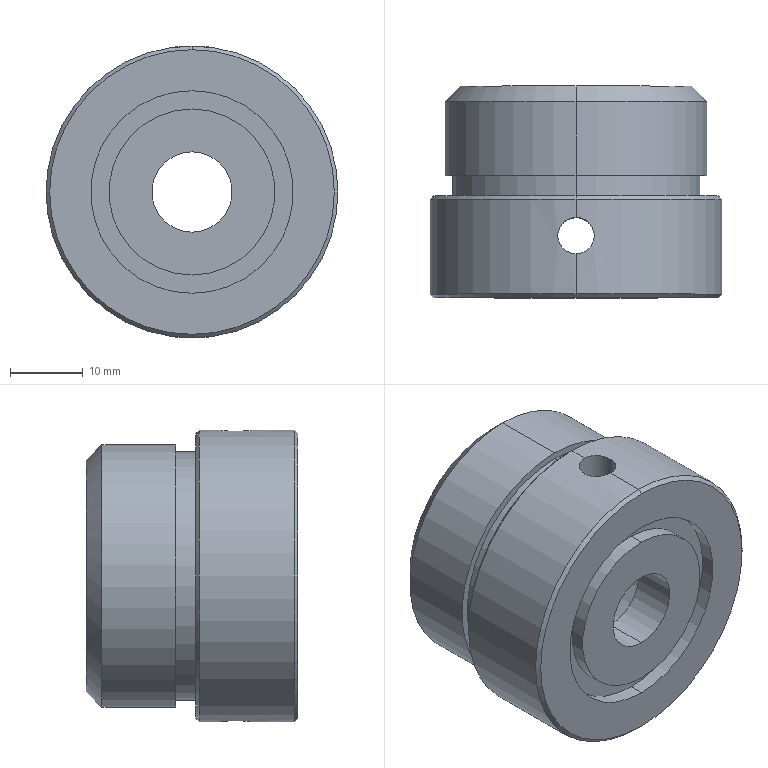Part | SolidWorks | features ICE 6, Chamfer 1, Extrusion 1, StudWizard 1 | 1 solid | 31 faces | box 40 x 29 x 40 mm | volume 19721 mm3 | cylinder 18 | plane 7 | cone 6 | commonest cylinder face diameters 5 x4 11 x2 22.75 x2 25 x2 27.75 x2 34 x2
STEP:
#1=CARTESIAN_POINT('',(0.,0.,-11.375));
#2=VERTEX_POINT('',#1);
#3=CARTESIAN_POINT('',(0.,0.,11.375));
#4=VERTEX_POINT('',#3);
#5=CARTESIAN_POINT('',(0.,0.,0.));
#6=DIRECTION('',(0.,-1.,0.));
#7=DIRECTION('',(0.,0.,1.));
#8=AXIS2_PLACEMENT_3D('',#5,#6,#7);
#9=CIRCLE('',#8,11.375);
#10=EDGE_CURVE('',#2,#4,#9,.T.);
#11=ORIENTED_EDGE('',*,*,#10,.F.);
#12=CARTESIAN_POINT('',(0.,2.,-11.375));
#13=VERTEX_POINT('',#12);
#14=CARTESIAN_POINT('',(0.,-0.000012,-11.375));
#15=DIRECTION('',(0.,1.,0.));
#16=VECTOR('',#15,1000.);
#17=LINE('',#14,#16);
#18=EDGE_CURVE('',#2,#13,#17,.T.);
#19=ORIENTED_EDGE('',*,*,#18,.T.);
#20=CARTESIAN_POINT('',(0.,2.,11.375));
#21=VERTEX_POINT('',#20);
#22=CARTESIAN_POINT('',(0.,2.,0.));
#23=DIRECTION('',(0.,-1.,0.));
#24=DIRECTION('',(0.,0.,-1.));
#25=AXIS2_PLACEMENT_3D('',#22,#23,#24);
#26=CIRCLE('',#25,11.375);
#27=EDGE_CURVE('',#13,#21,#26,.T.);
#28=ORIENTED_EDGE('',*,*,#27,.T.);
#29=CARTESIAN_POINT('',(0.,-0.000012,11.375));
#30=DIRECTION('',(0.,1.,0.));
#31=VECTOR('',#30,1000.);
#32=LINE('',#29,#31);
#33=EDGE_CURVE('',#4,#21,#32,.T.);
#34=ORIENTED_EDGE('',*,*,#33,.F.);
#35=EDGE_LOOP('',(#11,#19,#28,#34));
#36=FACE_OUTER_BOUND('',#35,.T.);
#37=CARTESIAN_POINT('',(0.,-0.000012,0.));
#38=DIRECTION('',(0.,1.,0.));
#39=DIRECTION('',(0.,0.,1.));
#40=AXIS2_PLACEMENT_3D('',#37,#38,#39);
#41=CYLINDRICAL_SURFACE('',#40,11.375);
#42=ADVANCED_FACE('',(#36),#41,.T.);
#43=CARTESIAN_POINT('',(0.,0.,13.875));
#44=VERTEX_POINT('',#43);
#45=CARTESIAN_POINT('',(0.,0.,-13.875));
#46=VERTEX_POINT('',#45);
#47=CARTESIAN_POINT('',(0.,0.,0.));
#48=DIRECTION('',(0.,-1.,0.));
#49=DIRECTION('',(0.,0.,1.));
#50=AXIS2_PLACEMENT_3D('',#47,#48,#49);
#51=CIRCLE('',#50,13.875);
#52=EDGE_CURVE('',#44,#46,#51,.T.);
#53=ORIENTED_EDGE('',*,*,#52,.T.);
#54=CARTESIAN_POINT('',(0.,2.,-13.875));
#55=VERTEX_POINT('',#54);
#56=CARTESIAN_POINT('',(0.,-0.000012,-13.875));
#57=DIRECTION('',(0.,1.,0.));
#58=VECTOR('',#57,1000.);
#59=LINE('',#56,#58);
#60=EDGE_CURVE('',#46,#55,#59,.T.);
#61=ORIENTED_EDGE('',*,*,#60,.T.);
#62=CARTESIAN_POINT('',(0.,2.,13.875));
#63=VERTEX_POINT('',#62);
#64=CARTESIAN_POINT('',(0.,2.,0.));
#65=DIRECTION('',(0.,-1.,0.));
#66=DIRECTION('',(0.,0.,-1.));
#67=AXIS2_PLACEMENT_3D('',#64,#65,#66);
#68=CIRCLE('',#67,13.875);
#69=EDGE_CURVE('',#63,#55,#68,.T.);
#70=ORIENTED_EDGE('',*,*,#69,.F.);
#71=CARTESIAN_POINT('',(0.,-0.000012,13.875));
#72=DIRECTION('',(0.,1.,0.));
#73=VECTOR('',#72,1000.);
#74=LINE('',#71,#73);
#75=EDGE_CURVE('',#44,#63,#74,.T.);
#76=ORIENTED_EDGE('',*,*,#75,.F.);
#77=EDGE_LOOP('',(#53,#61,#70,#76));
#78=FACE_OUTER_BOUND('',#77,.T.);
#79=CARTESIAN_POINT('',(0.,-0.000012,0.));
#80=DIRECTION('',(0.,1.,0.));
#81=DIRECTION('',(0.,0.,1.));
#82=AXIS2_PLACEMENT_3D('',#79,#80,#81);
#83=CYLINDRICAL_SURFACE('',#82,13.875);
#84=ADVANCED_FACE('',(#78),#83,.F.);
#85=CARTESIAN_POINT('',(0.,14.,19.5));
#86=VERTEX_POINT('',#85);
#87=CARTESIAN_POINT('',(0.,14.,-19.5));
#88=VERTEX_POINT('',#87);
#89=CARTESIAN_POINT('',(0.,14.,0.));
#90=DIRECTION('',(0.,1.,0.));
#91=DIRECTION('',(0.,0.,1.));
#92=AXIS2_PLACEMENT_3D('',#89,#90,#91);
#93=CIRCLE('',#92,19.5);
#94=EDGE_CURVE('',#86,#88,#93,.T.);
#95=ORIENTED_EDGE('',*,*,#94,.F.);
#96=CARTESIAN_POINT('',(0.,13.5,20.));
#97=VERTEX_POINT('',#96);
#98=CARTESIAN_POINT('',(0.,14.,19.5));
#99=DIRECTION('',(0.,-0.7071,0.7071));
#100=VECTOR('',#99,1000.);
#101=LINE('',#98,#100);
#102=EDGE_CURVE('',#86,#97,#101,.T.);
#103=ORIENTED_EDGE('',*,*,#102,.T.);
#104=CARTESIAN_POINT('',(0.,13.5,-20.));
#105=VERTEX_POINT('',#104);
#106=CARTESIAN_POINT('',(0.,13.5,0.));
#107=DIRECTION('',(0.,-1.,0.));
#108=DIRECTION('',(0.,0.,1.));
#109=AXIS2_PLACEMENT_3D('',#106,#107,#108);
#110=CIRCLE('',#109,20.);
#111=EDGE_CURVE('',#105,#97,#110,.T.);
#112=ORIENTED_EDGE('',*,*,#111,.F.);
#113=CARTESIAN_POINT('',(0.,14.,-19.5));
#114=DIRECTION('',(0.,-0.7071,-0.7071));
#115=VECTOR('',#114,1000.);
#116=LINE('',#113,#115);
#117=EDGE_CURVE('',#88,#105,#116,.T.);
#118=ORIENTED_EDGE('',*,*,#117,.F.);
#119=EDGE_LOOP('',(#95,#103,#112,#118));
#120=FACE_OUTER_BOUND('',#119,.T.);
#121=CARTESIAN_POINT('',(0.,14.,0.));
#122=DIRECTION('',(0.,-1.,0.));
#123=DIRECTION('',(0.,0.,-1.));
#124=AXIS2_PLACEMENT_3D('',#121,#122,#123);
#125=CONICAL_SURFACE('',#124,19.5,0.7854);
#126=ADVANCED_FACE('',(#120),#125,.T.);
#127=CARTESIAN_POINT('',(0.,0.,-19.5));
#128=VERTEX_POINT('',#127);
#129=CARTESIAN_POINT('',(0.,0.,19.5));
#130=VERTEX_POINT('',#129);
#131=CARTESIAN_POINT('',(0.,0.,0.));
#132=DIRECTION('',(0.,-1.,0.));
#133=DIRECTION('',(0.,0.,1.));
#134=AXIS2_PLACEMENT_3D('',#131,#132,#133);
#135=CIRCLE('',#134,19.5);
#136=EDGE_CURVE('',#128,#130,#135,.T.);
#137=ORIENTED_EDGE('',*,*,#136,.F.);
#138=CARTESIAN_POINT('',(0.,0.5,-20.));
#139=VERTEX_POINT('',#138);
#140=CARTESIAN_POINT('',(0.,0.5,-20.));
#141=DIRECTION('',(0.,0.7071,-0.7071));
#142=VECTOR('',#141,1000.);
#143=LINE('',#140,#142);
#144=EDGE_CURVE('',#128,#139,#143,.T.);
#145=ORIENTED_EDGE('',*,*,#144,.T.);
#146=CARTESIAN_POINT('',(0.,0.5,20.));
#147=VERTEX_POINT('',#146);
#148=CARTESIAN_POINT('',(0.,0.5,0.));
#149=DIRECTION('',(0.,1.,0.));
#150=DIRECTION('',(0.,0.,1.));
#151=AXIS2_PLACEMENT_3D('',#148,#149,#150);
#152=CIRCLE('',#151,20.);
#153=EDGE_CURVE('',#147,#139,#152,.T.);
#154=ORIENTED_EDGE('',*,*,#153,.F.);
#155=CARTESIAN_POINT('',(0.,0.5,20.));
#156=DIRECTION('',(0.,0.7071,0.7071));
#157=VECTOR('',#156,1000.);
#158=LINE('',#155,#157);
#159=EDGE_CURVE('',#130,#147,#158,.T.);
#160=ORIENTED_EDGE('',*,*,#159,.F.);
#161=EDGE_LOOP('',(#137,#145,#154,#160));
#162=FACE_OUTER_BOUND('',#161,.T.);
#163=CARTESIAN_POINT('',(0.,0.5,0.));
#164=DIRECTION('',(0.,1.,0.));
#165=DIRECTION('',(0.,0.,1.));
#166=AXIS2_PLACEMENT_3D('',#163,#164,#165);
#167=CONICAL_SURFACE('',#166,20.,0.7854);
#168=ADVANCED_FACE('',(#162),#167,.T.);
#169=CARTESIAN_POINT('',(0.,6.,-5.5));
#170=VERTEX_POINT('',#169);
#171=CARTESIAN_POINT('',(0.,6.,5.5));
#172=VERTEX_POINT('',#171);
#173=CARTESIAN_POINT('',(0.,6.,0.));
#174=DIRECTION('',(0.,1.,0.));
#175=DIRECTION('',(0.,0.,1.));
#176=AXIS2_PLACEMENT_3D('',#173,#174,#175);
#177=CIRCLE('',#176,5.5);
#178=EDGE_CURVE('',#170,#172,#177,.T.);
#179=ORIENTED_EDGE('',*,*,#178,.T.);
#180=CARTESIAN_POINT('',(0.,0.,5.5));
#181=VERTEX_POINT('',#180);
#182=CARTESIAN_POINT('',(0.,29.,5.5));
#183=DIRECTION('',(0.,-1.,0.));
#184=VECTOR('',#183,1000.);
#185=LINE('',#182,#184);
#186=EDGE_CURVE('',#172,#181,#185,.T.);
#187=ORIENTED_EDGE('',*,*,#186,.T.);
#188=CARTESIAN_POINT('',(0.,0.,-5.5));
#189=VERTEX_POINT('',#188);
#190=CARTESIAN_POINT('',(0.,0.,0.));
#191=DIRECTION('',(0.,1.,0.));
#192=DIRECTION('',(0.,0.,1.));
#193=AXIS2_PLACEMENT_3D('',#190,#191,#192);
#194=CIRCLE('',#193,5.5);
#195=EDGE_CURVE('',#189,#181,#194,.T.);
#196=ORIENTED_EDGE('',*,*,#195,.F.);
#197=CARTESIAN_POINT('',(0.,29.,-5.5));
#198=DIRECTION('',(0.,-1.,0.));
#199=VECTOR('',#198,1000.);
#200=LINE('',#197,#199);
#201=EDGE_CURVE('',#170,#189,#200,.T.);
#202=ORIENTED_EDGE('',*,*,#201,.F.);
#203=EDGE_LOOP('',(#179,#187,#196,#202));
#204=FACE_OUTER_BOUND('',#203,.T.);
#205=CARTESIAN_POINT('',(0.,29.,0.));
#206=DIRECTION('',(0.,-1.,0.));
#207=DIRECTION('',(0.,0.,-1.));
#208=AXIS2_PLACEMENT_3D('',#205,#206,#207);
#209=CYLINDRICAL_SURFACE('',#208,5.5);
#210=ADVANCED_FACE('',(#204),#209,.F.);
#211=CARTESIAN_POINT('',(-2.5,8.5,12.247));
#212=VERTEX_POINT('',#211);
#213=CARTESIAN_POINT('',(0.,6.,12.5));
#214=VERTEX_POINT('',#213);
#215=CARTESIAN_POINT('',(-2.5,8.5,12.247));
#216=CARTESIAN_POINT('',(-2.5,8.335,12.247));
#217=CARTESIAN_POINT('',(-2.484,8.172,12.251));
#218=CARTESIAN_POINT('',(-2.42,7.852,12.264));
#219=CARTESIAN_POINT('',(-2.372,7.693,12.273));
#220=CARTESIAN_POINT('',(-2.247,7.391,12.297));
#221=CARTESIAN_POINT('',(-2.17,7.248,12.311));
#222=CARTESIAN_POINT('',(-1.988,6.976,12.341));
#223=CARTESIAN_POINT('',(-1.883,6.848,12.358));
#224=CARTESIAN_POINT('',(-1.539,6.503,12.407));
#225=CARTESIAN_POINT('',(-1.261,6.317,12.44));
#226=CARTESIAN_POINT('',(-0.81,6.129,12.475));
#227=CARTESIAN_POINT('',(-0.6515,6.081,12.484));
#228=CARTESIAN_POINT('',(-0.3289,6.016,12.497));
#229=CARTESIAN_POINT('',(-0.1655,6.,12.5));
#230=CARTESIAN_POINT('',(0.,6.,12.5));
#231=B_SPLINE_CURVE_WITH_KNOTS('',3,(#215,#216,#217,#218,#219,#220,#221,#222,#223,#224,#225,#226,#227,#228,#229,#230),.UNSPECIFIED.,.F.,.F.,(4,2,2,2,2,2,2,4),(0.01175,0.01224,0.01273,0.01322,0.01371,0.01469,0.01518,0.01567),.UNSPECIFIED.);
#232=EDGE_CURVE('',#212,#214,#231,.T.);
#233=ORIENTED_EDGE('',*,*,#232,.F.);
#234=CARTESIAN_POINT('',(-2.5,8.5,19.843));
#235=VERTEX_POINT('',#234);
#236=CARTESIAN_POINT('',(-2.5,8.5,-20.));
#237=DIRECTION('',(0.,0.,1.));
#238=VECTOR('',#237,1000.);
#239=LINE('',#236,#238);
#240=EDGE_CURVE('',#212,#235,#239,.T.);
#241=ORIENTED_EDGE('',*,*,#240,.T.);
#242=CARTESIAN_POINT('',(0.,6.,20.));
#243=VERTEX_POINT('',#242);
#244=CARTESIAN_POINT('',(0.,6.,20.));
#245=CARTESIAN_POINT('',(-0.1632,6.,20.));
#246=CARTESIAN_POINT('',(-0.329,6.016,19.998));
#247=CARTESIAN_POINT('',(-0.6497,6.08,19.99));
#248=CARTESIAN_POINT('',(-0.8055,6.128,19.984));
#249=CARTESIAN_POINT('',(-1.108,6.253,19.97));
#250=CARTESIAN_POINT('',(-1.254,6.331,19.961));
#251=CARTESIAN_POINT('',(-1.525,6.512,19.942));
#252=CARTESIAN_POINT('',(-1.651,6.616,19.932));
#253=CARTESIAN_POINT('',(-1.884,6.849,19.911));
#254=CARTESIAN_POINT('',(-1.988,6.975,19.901));
#255=CARTESIAN_POINT('',(-2.169,7.246,19.882));
#256=CARTESIAN_POINT('',(-2.247,7.392,19.873));
#257=CARTESIAN_POINT('',(-2.372,7.695,19.859));
#258=CARTESIAN_POINT('',(-2.42,7.85,19.853));
#259=CARTESIAN_POINT('',(-2.484,8.171,19.845));
#260=CARTESIAN_POINT('',(-2.5,8.337,19.843));
#261=CARTESIAN_POINT('',(-2.5,8.5,19.843));
#262=B_SPLINE_CURVE_WITH_KNOTS('',3,(#244,#245,#246,#247,#248,#249,#250,#251,#252,#253,#254,#255,#256,#257,#258,#259,#260,#261),.UNSPECIFIED.,.F.,.F.,(4,2,2,2,2,2,2,2,4),(0.003913,0.004402,0.004891,0.005379,0.005868,0.006357,0.006846,0.007335,0.007824),.UNSPECIFIED.);
#263=EDGE_CURVE('',#243,#235,#262,.T.);
#264=ORIENTED_EDGE('',*,*,#263,.F.);
#265=CARTESIAN_POINT('',(2.5,8.5,19.843));
#266=VERTEX_POINT('',#265);
#267=CARTESIAN_POINT('',(2.5,8.5,19.843));
#268=CARTESIAN_POINT('',(2.5,8.335,19.843));
#269=CARTESIAN_POINT('',(2.484,8.172,19.845));
#270=CARTESIAN_POINT('',(2.42,7.852,19.853));
#271=CARTESIAN_POINT('',(2.372,7.693,19.859));
#272=CARTESIAN_POINT('',(2.246,7.391,19.874));
#273=CARTESIAN_POINT('',(2.169,7.247,19.882));
#274=CARTESIAN_POINT('',(1.988,6.975,19.901));
#275=CARTESIAN_POINT('',(1.882,6.847,19.912));
#276=CARTESIAN_POINT('',(1.652,6.616,19.932));
#277=CARTESIAN_POINT('',(1.526,6.513,19.942));
#278=CARTESIAN_POINT('',(1.253,6.33,19.961));
#279=CARTESIAN_POINT('',(1.107,6.253,19.97));
#280=CARTESIAN_POINT('',(0.8064,6.128,19.984));
#281=CARTESIAN_POINT('',(0.6486,6.08,19.99));
#282=CARTESIAN_POINT('',(0.3257,6.016,19.998));
#283=CARTESIAN_POINT('',(0.1633,6.,20.));
#284=CARTESIAN_POINT('',(0.,6.,20.));
#285=B_SPLINE_CURVE_WITH_KNOTS('',3,(#267,#268,#269,#270,#271,#272,#273,#274,#275,#276,#277,#278,#279,#280,#281,#282,#283,#284),.UNSPECIFIED.,.F.,.F.,(4,2,2,2,2,2,2,2,4),(0.,0.0004891,0.0009782,0.001467,0.001956,0.002446,0.002935,0.003424,0.003913),.UNSPECIFIED.);
#286=EDGE_CURVE('',#266,#243,#285,.T.);
#287=ORIENTED_EDGE('',*,*,#286,.F.);
#288=CARTESIAN_POINT('',(2.5,8.5,12.247));
#289=VERTEX_POINT('',#288);
#290=CARTESIAN_POINT('',(2.5,8.5,-20.));
#291=DIRECTION('',(0.,0.,1.));
#292=VECTOR('',#291,1000.);
#293=LINE('',#290,#292);
#294=EDGE_CURVE('',#289,#266,#293,.T.);
#295=ORIENTED_EDGE('',*,*,#294,.F.);
#296=CARTESIAN_POINT('',(0.,6.,12.5));
#297=CARTESIAN_POINT('',(0.1657,6.,12.5));
#298=CARTESIAN_POINT('',(0.3285,6.016,12.497));
#299=CARTESIAN_POINT('',(0.6487,6.08,12.484));
#300=CARTESIAN_POINT('',(0.8078,6.128,12.475));
#301=CARTESIAN_POINT('',(1.11,6.254,12.452));
#302=CARTESIAN_POINT('',(1.254,6.331,12.438));
#303=CARTESIAN_POINT('',(1.525,6.513,12.407));
#304=CARTESIAN_POINT('',(1.654,6.618,12.391));
#305=CARTESIAN_POINT('',(1.999,6.963,12.341));
#306=CARTESIAN_POINT('',(2.185,7.242,12.308));
#307=CARTESIAN_POINT('',(2.372,7.693,12.273));
#308=CARTESIAN_POINT('',(2.42,7.851,12.264));
#309=CARTESIAN_POINT('',(2.484,8.174,12.251));
#310=CARTESIAN_POINT('',(2.5,8.336,12.247));
#311=CARTESIAN_POINT('',(2.5,8.5,12.247));
#312=B_SPLINE_CURVE_WITH_KNOTS('',3,(#296,#297,#298,#299,#300,#301,#302,#303,#304,#305,#306,#307,#308,#309,#310,#311),.UNSPECIFIED.,.F.,.F.,(4,2,2,2,2,2,2,4),(0.,0.0004899,0.0009797,0.00147,0.001959,0.002939,0.003429,0.003919),.UNSPECIFIED.);
#313=EDGE_CURVE('',#214,#289,#312,.T.);
#314=ORIENTED_EDGE('',*,*,#313,.F.);
#315=EDGE_LOOP('',(#233,#241,#264,#287,#295,#314));
#316=FACE_OUTER_BOUND('',#315,.T.);
#317=CARTESIAN_POINT('',(0.,8.5,-20.));
#318=DIRECTION('',(0.,0.,1.));
#319=DIRECTION('',(1.,0.,0.));
#320=AXIS2_PLACEMENT_3D('',#317,#318,#319);
#321=CYLINDRICAL_SURFACE('',#320,2.5);
#322=ADVANCED_FACE('',(#316),#321,.F.);
#323=CARTESIAN_POINT('',(-2.5,8.5,-19.843));
#324=VERTEX_POINT('',#323);
#325=CARTESIAN_POINT('',(0.,6.,-20.));
#326=VERTEX_POINT('',#325);
#327=CARTESIAN_POINT('',(-2.5,8.5,-19.843));
#328=CARTESIAN_POINT('',(-2.5,8.337,-19.843));
#329=CARTESIAN_POINT('',(-2.484,8.171,-19.845));
#330=CARTESIAN_POINT('',(-2.42,7.85,-19.853));
#331=CARTESIAN_POINT('',(-2.372,7.694,-19.859));
#332=CARTESIAN_POINT('',(-2.247,7.392,-19.873));
#333=CARTESIAN_POINT('',(-2.169,7.246,-19.882));
#334=CARTESIAN_POINT('',(-1.988,6.975,-19.901));
#335=CARTESIAN_POINT('',(-1.884,6.849,-19.911));
#336=CARTESIAN_POINT('',(-1.651,6.616,-19.932));
#337=CARTESIAN_POINT('',(-1.525,6.512,-19.942));
#338=CARTESIAN_POINT('',(-1.254,6.331,-19.961));
#339=CARTESIAN_POINT('',(-1.108,6.253,-19.97));
#340=CARTESIAN_POINT('',(-0.8055,6.128,-19.984));
#341=CARTESIAN_POINT('',(-0.6496,6.08,-19.99));
#342=CARTESIAN_POINT('',(-0.329,6.016,-19.998));
#343=CARTESIAN_POINT('',(-0.1632,6.,-20.));
#344=CARTESIAN_POINT('',(0.,6.,-20.));
#345=B_SPLINE_CURVE_WITH_KNOTS('',3,(#327,#328,#329,#330,#331,#332,#333,#334,#335,#336,#337,#338,#339,#340,#341,#342,#343,#344),.UNSPECIFIED.,.F.,.F.,(4,2,2,2,2,2,2,2,4),(0.003913,0.004402,0.004891,0.005379,0.005868,0.006357,0.006846,0.007335,0.007824),.UNSPECIFIED.);
#346=EDGE_CURVE('',#324,#326,#345,.T.);
#347=ORIENTED_EDGE('',*,*,#346,.F.);
#348=CARTESIAN_POINT('',(-2.5,8.5,-12.247));
#349=VERTEX_POINT('',#348);
#350=CARTESIAN_POINT('',(-2.5,8.5,-20.));
#351=DIRECTION('',(0.,0.,1.));
#352=VECTOR('',#351,1000.);
#353=LINE('',#350,#352);
#354=EDGE_CURVE('',#324,#349,#353,.T.);
#355=ORIENTED_EDGE('',*,*,#354,.T.);
#356=CARTESIAN_POINT('',(0.,6.,-12.5));
#357=VERTEX_POINT('',#356);
#358=CARTESIAN_POINT('',(0.,6.,-12.5));
#359=CARTESIAN_POINT('',(-0.1657,6.,-12.5));
#360=CARTESIAN_POINT('',(-0.3285,6.016,-12.497));
#361=CARTESIAN_POINT('',(-0.6487,6.08,-12.484));
#362=CARTESIAN_POINT('',(-0.8078,6.128,-12.475));
#363=CARTESIAN_POINT('',(-1.11,6.254,-12.452));
#364=CARTESIAN_POINT('',(-1.254,6.331,-12.438));
#365=CARTESIAN_POINT('',(-1.525,6.513,-12.407));
#366=CARTESIAN_POINT('',(-1.654,6.618,-12.391));
#367=CARTESIAN_POINT('',(-1.999,6.963,-12.341));
#368=CARTESIAN_POINT('',(-2.185,7.242,-12.308));
#369=CARTESIAN_POINT('',(-2.372,7.693,-12.273));
#370=CARTESIAN_POINT('',(-2.42,7.851,-12.264));
#371=CARTESIAN_POINT('',(-2.484,8.174,-12.251));
#372=CARTESIAN_POINT('',(-2.5,8.336,-12.247));
#373=CARTESIAN_POINT('',(-2.5,8.5,-12.247));
#374=B_SPLINE_CURVE_WITH_KNOTS('',3,(#358,#359,#360,#361,#362,#363,#364,#365,#366,#367,#368,#369,#370,#371,#372,#373),.UNSPECIFIED.,.F.,.F.,(4,2,2,2,2,2,2,4),(0.,0.0004899,0.0009797,0.00147,0.001959,0.002939,0.003429,0.003919),.UNSPECIFIED.);
#375=EDGE_CURVE('',#357,#349,#374,.T.);
#376=ORIENTED_EDGE('',*,*,#375,.F.);
#377=CARTESIAN_POINT('',(2.5,8.5,-12.247));
#378=VERTEX_POINT('',#377);
#379=CARTESIAN_POINT('',(2.5,8.5,-12.247));
#380=CARTESIAN_POINT('',(2.5,8.335,-12.247));
#381=CARTESIAN_POINT('',(2.484,8.172,-12.251));
#382=CARTESIAN_POINT('',(2.42,7.852,-12.264));
#383=CARTESIAN_POINT('',(2.372,7.693,-12.273));
#384=CARTESIAN_POINT('',(2.247,7.391,-12.297));
#385=CARTESIAN_POINT('',(2.17,7.248,-12.311));
#386=CARTESIAN_POINT('',(1.988,6.976,-12.341));
#387=CARTESIAN_POINT('',(1.883,6.848,-12.358));
#388=CARTESIAN_POINT('',(1.539,6.503,-12.407));
#389=CARTESIAN_POINT('',(1.261,6.317,-12.44));
#390=CARTESIAN_POINT('',(0.81,6.129,-12.475));
#391=CARTESIAN_POINT('',(0.6515,6.081,-12.484));
#392=CARTESIAN_POINT('',(0.3289,6.016,-12.497));
#393=CARTESIAN_POINT('',(0.1655,6.,-12.5));
#394=CARTESIAN_POINT('',(0.,6.,-12.5));
#395=B_SPLINE_CURVE_WITH_KNOTS('',3,(#379,#380,#381,#382,#383,#384,#385,#386,#387,#388,#389,#390,#391,#392,#393,#394),.UNSPECIFIED.,.F.,.F.,(4,2,2,2,2,2,2,4),(0.01175,0.01224,0.01273,0.01322,0.01371,0.01469,0.01518,0.01567),.UNSPECIFIED.);
#396=EDGE_CURVE('',#378,#357,#395,.T.);
#397=ORIENTED_EDGE('',*,*,#396,.F.);
#398=CARTESIAN_POINT('',(2.5,8.5,-19.843));
#399=VERTEX_POINT('',#398);
#400=CARTESIAN_POINT('',(2.5,8.5,-20.));
#401=DIRECTION('',(0.,0.,1.));
#402=VECTOR('',#401,1000.);
#403=LINE('',#400,#402);
#404=EDGE_CURVE('',#399,#378,#403,.T.);
#405=ORIENTED_EDGE('',*,*,#404,.F.);
#406=CARTESIAN_POINT('',(0.,6.,-20.));
#407=CARTESIAN_POINT('',(0.1633,6.,-20.));
#408=CARTESIAN_POINT('',(0.3257,6.016,-19.998));
#409=CARTESIAN_POINT('',(0.6486,6.08,-19.99));
#410=CARTESIAN_POINT('',(0.8064,6.128,-19.984));
#411=CARTESIAN_POINT('',(1.107,6.253,-19.97));
#412=CARTESIAN_POINT('',(1.253,6.33,-19.961));
#413=CARTESIAN_POINT('',(1.526,6.513,-19.942));
#414=CARTESIAN_POINT('',(1.652,6.616,-19.932));
#415=CARTESIAN_POINT('',(1.883,6.847,-19.912));
#416=CARTESIAN_POINT('',(1.988,6.975,-19.901));
#417=CARTESIAN_POINT('',(2.169,7.247,-19.882));
#418=CARTESIAN_POINT('',(2.246,7.391,-19.874));
#419=CARTESIAN_POINT('',(2.372,7.693,-19.859));
#420=CARTESIAN_POINT('',(2.42,7.852,-19.853));
#421=CARTESIAN_POINT('',(2.484,8.172,-19.845));
#422=CARTESIAN_POINT('',(2.5,8.335,-19.843));
#423=CARTESIAN_POINT('',(2.5,8.5,-19.843));
#424=B_SPLINE_CURVE_WITH_KNOTS('',3,(#406,#407,#408,#409,#410,#411,#412,#413,#414,#415,#416,#417,#418,#419,#420,#421,#422,#423),.UNSPECIFIED.,.F.,.F.,(4,2,2,2,2,2,2,2,4),(0.007824,0.008313,0.008802,0.009291,0.00978,0.01027,0.01076,0.01125,0.01174),.UNSPECIFIED.);
#425=EDGE_CURVE('',#326,#399,#424,.T.);
#426=ORIENTED_EDGE('',*,*,#425,.F.);
#427=EDGE_LOOP('',(#347,#355,#376,#397,#405,#426));
#428=FACE_OUTER_BOUND('',#427,.T.);
#429=CARTESIAN_POINT('',(0.,8.5,-20.));
#430=DIRECTION('',(0.,0.,1.));
#431=DIRECTION('',(1.,0.,0.));
#432=AXIS2_PLACEMENT_3D('',#429,#430,#431);
#433=CYLINDRICAL_SURFACE('',#432,2.5);
#434=ADVANCED_FACE('',(#428),#433,.F.);
#435=ORIENTED_EDGE('',*,*,#375,.T.);
#436=CARTESIAN_POINT('',(0.,11.,-12.5));
#437=VERTEX_POINT('',#436);
#438=CARTESIAN_POINT('',(-2.5,8.5,-12.247));
#439=CARTESIAN_POINT('',(-2.5,8.663,-12.247));
#440=CARTESIAN_POINT('',(-2.484,8.83,-12.251));
#441=CARTESIAN_POINT('',(-2.419,9.15,-12.264));
#442=CARTESIAN_POINT('',(-2.372,9.306,-12.273));
#443=CARTESIAN_POINT('',(-2.246,9.61,-12.297));
#444=CARTESIAN_POINT('',(-2.168,9.755,-12.311));
#445=CARTESIAN_POINT('',(-1.987,10.025,-12.341));
#446=CARTESIAN_POINT('',(-1.883,10.152,-12.358));
#447=CARTESIAN_POINT('',(-1.651,10.384,-12.391));
#448=CARTESIAN_POINT('',(-1.525,10.487,-12.407));
#449=CARTESIAN_POINT('',(-1.255,10.668,-12.438));
#450=CARTESIAN_POINT('',(-1.109,10.747,-12.452));
#451=CARTESIAN_POINT('',(-0.8064,10.872,-12.475));
#452=CARTESIAN_POINT('',(-0.6505,10.919,-12.484));
#453=CARTESIAN_POINT('',(-0.3293,10.984,-12.497));
#454=CARTESIAN_POINT('',(-0.1633,11.,-12.5));
#455=CARTESIAN_POINT('',(0.,11.,-12.5));
#456=B_SPLINE_CURVE_WITH_KNOTS('',3,(#438,#439,#440,#441,#442,#443,#444,#445,#446,#447,#448,#449,#450,#451,#452,#453,#454,#455),.UNSPECIFIED.,.F.,.F.,(4,2,2,2,2,2,2,2,4),(0.003919,0.004409,0.004898,0.005388,0.005877,0.006367,0.006857,0.007346,0.007836),.UNSPECIFIED.);
#457=EDGE_CURVE('',#349,#437,#456,.T.);
#458=ORIENTED_EDGE('',*,*,#457,.T.);
#459=CARTESIAN_POINT('',(0.,29.,-12.5));
#460=VERTEX_POINT('',#459);
#461=CARTESIAN_POINT('',(0.,6.,-12.5));
#462=DIRECTION('',(0.,1.,0.));
#463=VECTOR('',#462,1000.);
#464=LINE('',#461,#463);
#465=EDGE_CURVE('',#437,#460,#464,.T.);
#466=ORIENTED_EDGE('',*,*,#465,.T.);
#467=CARTESIAN_POINT('',(0.,29.,12.5));
#468=VERTEX_POINT('',#467);
#469=CARTESIAN_POINT('',(0.,29.,0.));
#470=DIRECTION('',(0.,1.,0.));
#471=DIRECTION('',(0.,0.,1.));
#472=AXIS2_PLACEMENT_3D('',#469,#470,#471);
#473=CIRCLE('',#472,12.5);
#474=EDGE_CURVE('',#460,#468,#473,.T.);
#475=ORIENTED_EDGE('',*,*,#474,.T.);
#476=CARTESIAN_POINT('',(0.,11.,12.5));
#477=VERTEX_POINT('',#476);
#478=CARTESIAN_POINT('',(0.,6.,12.5));
#479=DIRECTION('',(0.,1.,0.));
#480=VECTOR('',#479,1000.);
#481=LINE('',#478,#480);
#482=EDGE_CURVE('',#477,#468,#481,.T.);
#483=ORIENTED_EDGE('',*,*,#482,.F.);
#484=CARTESIAN_POINT('',(0.,11.,12.5));
#485=CARTESIAN_POINT('',(-0.3268,11.,12.5));
#486=CARTESIAN_POINT('',(-0.6566,10.934,12.486));
#487=CARTESIAN_POINT('',(-1.108,10.747,12.452));
#488=CARTESIAN_POINT('',(-1.254,10.669,12.438));
#489=CARTESIAN_POINT('',(-1.526,10.487,12.407));
#490=CARTESIAN_POINT('',(-1.652,10.384,12.391));
#491=CARTESIAN_POINT('',(-1.882,10.153,12.358));
#492=CARTESIAN_POINT('',(-1.988,10.025,12.341));
#493=CARTESIAN_POINT('',(-2.169,9.754,12.311));
#494=CARTESIAN_POINT('',(-2.246,9.611,12.297));
#495=CARTESIAN_POINT('',(-2.435,9.155,12.261));
#496=CARTESIAN_POINT('',(-2.5,8.83,12.247));
#497=CARTESIAN_POINT('',(-2.5,8.5,12.247));
#498=B_SPLINE_CURVE_WITH_KNOTS('',3,(#484,#485,#486,#487,#488,#489,#490,#491,#492,#493,#494,#495,#496,#497),.UNSPECIFIED.,.F.,.F.,(4,2,2,2,2,2,4),(0.007836,0.008815,0.009305,0.009795,0.01028,0.01077,0.01175),.UNSPECIFIED.);
#499=EDGE_CURVE('',#477,#212,#498,.T.);
#500=ORIENTED_EDGE('',*,*,#499,.T.);
#501=ORIENTED_EDGE('',*,*,#232,.T.);
#502=CARTESIAN_POINT('',(0.,6.,0.));
#503=DIRECTION('',(0.,1.,0.));
#504=DIRECTION('',(0.,0.,1.));
#505=AXIS2_PLACEMENT_3D('',#502,#503,#504);
#506=CIRCLE('',#505,12.5);
#507=EDGE_CURVE('',#357,#214,#506,.T.);
#508=ORIENTED_EDGE('',*,*,#507,.F.);
#509=EDGE_LOOP('',(#435,#458,#466,#475,#483,#500,#501,#508));
#510=FACE_OUTER_BOUND('',#509,.T.);
#511=CARTESIAN_POINT('',(0.,6.,0.));
#512=DIRECTION('',(0.,1.,0.));
#513=DIRECTION('',(0.,0.,1.));
#514=AXIS2_PLACEMENT_3D('',#511,#512,#513);
#515=CYLINDRICAL_SURFACE('',#514,12.5);
#516=ADVANCED_FACE('',(#510),#515,.F.);
#517=CARTESIAN_POINT('',(0.,29.,-15.835));
#518=VERTEX_POINT('',#517);
#519=CARTESIAN_POINT('',(0.,29.,15.835));
#520=VERTEX_POINT('',#519);
#521=CARTESIAN_POINT('',(0.,29.,0.));
#522=DIRECTION('',(0.,-1.,0.));
#523=DIRECTION('',(0.,0.,-1.));
#524=AXIS2_PLACEMENT_3D('',#521,#522,#523);
#525=CIRCLE('',#524,15.835);
#526=EDGE_CURVE('',#518,#520,#525,.T.);
#527=ORIENTED_EDGE('',*,*,#526,.T.);
#528=CARTESIAN_POINT('',(0.,26.835,18.));
#529=VERTEX_POINT('',#528);
#530=CARTESIAN_POINT('',(0.,29.,15.835));
#531=DIRECTION('',(0.,-0.7071,0.7071));
#532=VECTOR('',#531,1000.);
#533=LINE('',#530,#532);
#534=EDGE_CURVE('',#520,#529,#533,.T.);
#535=ORIENTED_EDGE('',*,*,#534,.T.);
#536=CARTESIAN_POINT('',(0.,26.835,-18.));
#537=VERTEX_POINT('',#536);
#538=CARTESIAN_POINT('',(0.,26.835,0.));
#539=DIRECTION('',(0.,-1.,0.));
#540=DIRECTION('',(0.,0.,-1.));
#541=AXIS2_PLACEMENT_3D('',#538,#539,#540);
#542=CIRCLE('',#541,18.);
#543=EDGE_CURVE('',#537,#529,#542,.T.);
#544=ORIENTED_EDGE('',*,*,#543,.F.);
#545=CARTESIAN_POINT('',(0.,29.,-15.835));
#546=DIRECTION('',(0.,-0.7071,-0.7071));
#547=VECTOR('',#546,1000.);
#548=LINE('',#545,#547);
#549=EDGE_CURVE('',#518,#537,#548,.T.);
#550=ORIENTED_EDGE('',*,*,#549,.F.);
#551=EDGE_LOOP('',(#527,#535,#544,#550));
#552=FACE_OUTER_BOUND('',#551,.T.);
#553=CARTESIAN_POINT('',(0.,29.,0.));
#554=DIRECTION('',(0.,-1.,0.));
#555=DIRECTION('',(0.,0.,-1.));
#556=AXIS2_PLACEMENT_3D('',#553,#554,#555);
#557=CONICAL_SURFACE('',#556,15.835,0.7854);
#558=ADVANCED_FACE('',(#552),#557,.T.);
#559=ORIENTED_EDGE('',*,*,#543,.T.);
#560=CARTESIAN_POINT('',(0.,16.75,18.));
#561=VERTEX_POINT('',#560);
#562=CARTESIAN_POINT('',(0.,29.,18.));
#563=DIRECTION('',(0.,-1.,0.));
#564=VECTOR('',#563,1000.);
#565=LINE('',#562,#564);
#566=EDGE_CURVE('',#529,#561,#565,.T.);
#567=ORIENTED_EDGE('',*,*,#566,.T.);
#568=CARTESIAN_POINT('',(0.,16.75,-18.));
#569=VERTEX_POINT('',#568);
#570=CARTESIAN_POINT('',(0.,16.75,0.));
#571=DIRECTION('',(0.,-1.,0.));
#572=DIRECTION('',(0.,0.,-1.));
#573=AXIS2_PLACEMENT_3D('',#570,#571,#572);
#574=CIRCLE('',#573,18.);
#575=EDGE_CURVE('',#569,#561,#574,.T.);
#576=ORIENTED_EDGE('',*,*,#575,.F.);
#577=CARTESIAN_POINT('',(0.,29.,-18.));
#578=DIRECTION('',(0.,-1.,0.));
#579=VECTOR('',#578,1000.);
#580=LINE('',#577,#579);
#581=EDGE_CURVE('',#537,#569,#580,.T.);
#582=ORIENTED_EDGE('',*,*,#581,.F.);
#583=EDGE_LOOP('',(#559,#567,#576,#582));
#584=FACE_OUTER_BOUND('',#583,.T.);
#585=CARTESIAN_POINT('',(0.,29.,0.));
#586=DIRECTION('',(0.,-1.,0.));
#587=DIRECTION('',(0.,0.,-1.));
#588=AXIS2_PLACEMENT_3D('',#585,#586,#587);
#589=CYLINDRICAL_SURFACE('',#588,18.);
#590=ADVANCED_FACE('',(#584),#589,.T.);
#591=CARTESIAN_POINT('',(0.,16.75,17.));
#592=VERTEX_POINT('',#591);
#593=CARTESIAN_POINT('',(0.,16.75,-17.));
#594=VERTEX_POINT('',#593);
#595=CARTESIAN_POINT('',(0.,16.75,0.));
#596=DIRECTION('',(0.,1.,0.));
#597=DIRECTION('',(0.,0.,1.));
#598=AXIS2_PLACEMENT_3D('',#595,#596,#597);
#599=CIRCLE('',#598,17.);
#600=EDGE_CURVE('',#592,#594,#599,.T.);
#601=ORIENTED_EDGE('',*,*,#600,.F.);
#602=CARTESIAN_POINT('',(0.,14.,17.));
#603=VERTEX_POINT('',#602);
#604=CARTESIAN_POINT('',(0.,16.75,17.));
#605=DIRECTION('',(0.,-1.,0.));
#606=VECTOR('',#605,1000.);
#607=LINE('',#604,#606);
#608=EDGE_CURVE('',#592,#603,#607,.T.);
#609=ORIENTED_EDGE('',*,*,#608,.T.);
#610=CARTESIAN_POINT('',(0.,14.,-17.));
#611=VERTEX_POINT('',#610);
#612=CARTESIAN_POINT('',(0.,14.,0.));
#613=DIRECTION('',(0.,1.,0.));
#614=DIRECTION('',(0.,0.,1.));
#615=AXIS2_PLACEMENT_3D('',#612,#613,#614);
#616=CIRCLE('',#615,17.);
#617=EDGE_CURVE('',#603,#611,#616,.T.);
#618=ORIENTED_EDGE('',*,*,#617,.T.);
#619=CARTESIAN_POINT('',(0.,16.75,-17.));
#620=DIRECTION('',(0.,-1.,0.));
#621=VECTOR('',#620,1000.);
#622=LINE('',#619,#621);
#623=EDGE_CURVE('',#594,#611,#622,.T.);
#624=ORIENTED_EDGE('',*,*,#623,.F.);
#625=EDGE_LOOP('',(#601,#609,#618,#624));
#626=FACE_OUTER_BOUND('',#625,.T.);
#627=CARTESIAN_POINT('',(0.,16.75,0.));
#628=DIRECTION('',(0.,-1.,0.));
#629=DIRECTION('',(0.,0.,-1.));
#630=AXIS2_PLACEMENT_3D('',#627,#628,#629);
#631=CYLINDRICAL_SURFACE('',#630,17.);
#632=ADVANCED_FACE('',(#626),#631,.T.);
#633=ORIENTED_EDGE('',*,*,#111,.T.);
#634=CARTESIAN_POINT('',(0.,11.,20.));
#635=VERTEX_POINT('',#634);
#636=CARTESIAN_POINT('',(0.,14.,20.));
#637=DIRECTION('',(0.,-1.,0.));
#638=VECTOR('',#637,1000.);
#639=LINE('',#636,#638);
#640=EDGE_CURVE('',#97,#635,#639,.T.);
#641=ORIENTED_EDGE('',*,*,#640,.T.);
#642=CARTESIAN_POINT('',(0.,11.,20.));
#643=CARTESIAN_POINT('',(0.1652,11.,20.));
#644=CARTESIAN_POINT('',(0.3276,10.984,19.998));
#645=CARTESIAN_POINT('',(0.6472,10.92,19.99));
#646=CARTESIAN_POINT('',(0.806,10.872,19.984));
#647=CARTESIAN_POINT('',(1.109,10.747,19.97));
#648=CARTESIAN_POINT('',(1.252,10.67,19.961));
#649=CARTESIAN_POINT('',(1.524,10.489,19.942));
#650=CARTESIAN_POINT('',(1.652,10.383,19.932));
#651=CARTESIAN_POINT('',(1.882,10.153,19.912));
#652=CARTESIAN_POINT('',(1.986,10.028,19.901));
#653=CARTESIAN_POINT('',(2.169,9.755,19.882));
#654=CARTESIAN_POINT('',(2.246,9.61,19.874));
#655=CARTESIAN_POINT('',(2.433,9.159,19.852));
#656=CARTESIAN_POINT('',(2.5,8.83,19.843));
#657=CARTESIAN_POINT('',(2.5,8.5,19.843));
#658=B_SPLINE_CURVE_WITH_KNOTS('',3,(#642,#643,#644,#645,#646,#647,#648,#649,#650,#651,#652,#653,#654,#655,#656,#657),.UNSPECIFIED.,.F.,.F.,(4,2,2,2,2,2,2,4),(0.01174,0.01223,0.01271,0.0132,0.01369,0.01418,0.01467,0.01565),.UNSPECIFIED.);
#659=EDGE_CURVE('',#635,#266,#658,.T.);
#660=ORIENTED_EDGE('',*,*,#659,.T.);
#661=ORIENTED_EDGE('',*,*,#286,.T.);
#662=CARTESIAN_POINT('',(0.,14.,20.));
#663=DIRECTION('',(0.,-1.,0.));
#664=VECTOR('',#663,1000.);
#665=LINE('',#662,#664);
#666=EDGE_CURVE('',#243,#147,#665,.T.);
#667=ORIENTED_EDGE('',*,*,#666,.T.);
#668=ORIENTED_EDGE('',*,*,#153,.T.);
#669=CARTESIAN_POINT('',(0.,14.,-20.));
#670=DIRECTION('',(0.,-1.,0.));
#671=VECTOR('',#670,1000.);
#672=LINE('',#669,#671);
#673=EDGE_CURVE('',#326,#139,#672,.T.);
#674=ORIENTED_EDGE('',*,*,#673,.F.);
#675=ORIENTED_EDGE('',*,*,#425,.T.);
#676=CARTESIAN_POINT('',(0.,11.,-20.));
#677=VERTEX_POINT('',#676);
#678=CARTESIAN_POINT('',(2.5,8.5,-19.843));
#679=CARTESIAN_POINT('',(2.5,8.665,-19.843));
#680=CARTESIAN_POINT('',(2.484,8.828,-19.845));
#681=CARTESIAN_POINT('',(2.42,9.147,-19.853));
#682=CARTESIAN_POINT('',(2.372,9.306,-19.859));
#683=CARTESIAN_POINT('',(2.247,9.609,-19.873));
#684=CARTESIAN_POINT('',(2.17,9.752,-19.882));
#685=CARTESIAN_POINT('',(1.989,10.024,-19.901));
#686=CARTESIAN_POINT('',(1.883,10.152,-19.911));
#687=CARTESIAN_POINT('',(1.653,10.382,-19.932));
#688=CARTESIAN_POINT('',(1.528,10.486,-19.942));
#689=CARTESIAN_POINT('',(1.255,10.669,-19.961));
#690=CARTESIAN_POINT('',(1.11,10.746,-19.97));
#691=CARTESIAN_POINT('',(0.6588,10.933,-19.991));
#692=CARTESIAN_POINT('',(0.3305,11.,-20.));
#693=CARTESIAN_POINT('',(0.,11.,-20.));
#694=B_SPLINE_CURVE_WITH_KNOTS('',3,(#678,#679,#680,#681,#682,#683,#684,#685,#686,#687,#688,#689,#690,#691,#692,#693),.UNSPECIFIED.,.F.,.F.,(4,2,2,2,2,2,2,4),(0.01174,0.01223,0.01271,0.0132,0.01369,0.01418,0.01467,0.01565),.UNSPECIFIED.);
#695=EDGE_CURVE('',#399,#677,#694,.T.);
#696=ORIENTED_EDGE('',*,*,#695,.T.);
#697=CARTESIAN_POINT('',(0.,14.,-20.));
#698=DIRECTION('',(0.,-1.,0.));
#699=VECTOR('',#698,1000.);
#700=LINE('',#697,#699);
#701=EDGE_CURVE('',#105,#677,#700,.T.);
#702=ORIENTED_EDGE('',*,*,#701,.F.);
#703=EDGE_LOOP('',(#633,#641,#660,#661,#667,#668,#674,#675,#696,#702));
#704=FACE_OUTER_BOUND('',#703,.T.);
#705=CARTESIAN_POINT('',(0.,14.,0.));
#706=DIRECTION('',(0.,-1.,0.));
#707=DIRECTION('',(0.,0.,-1.));
#708=AXIS2_PLACEMENT_3D('',#705,#706,#707);
#709=CYLINDRICAL_SURFACE('',#708,20.);
#710=ADVANCED_FACE('',(#704),#709,.T.);
#711=ORIENTED_EDGE('',*,*,#195,.T.);
#712=CARTESIAN_POINT('',(0.,0.,0.));
#713=DIRECTION('',(0.,1.,0.));
#714=DIRECTION('',(0.,0.,1.));
#715=AXIS2_PLACEMENT_3D('',#712,#713,#714);
#716=CIRCLE('',#715,5.5);
#717=EDGE_CURVE('',#181,#189,#716,.T.);
#718=ORIENTED_EDGE('',*,*,#717,.T.);
#719=EDGE_LOOP('',(#711,#718));
#720=FACE_BOUND('',#719,.T.);
#721=CARTESIAN_POINT('',(0.,0.,0.));
#722=DIRECTION('',(0.,-1.,0.));
#723=DIRECTION('',(0.,0.,1.));
#724=AXIS2_PLACEMENT_3D('',#721,#722,#723);
#725=CIRCLE('',#724,11.375);
#726=EDGE_CURVE('',#4,#2,#725,.T.);
#727=ORIENTED_EDGE('',*,*,#726,.T.);
#728=ORIENTED_EDGE('',*,*,#10,.T.);
#729=EDGE_LOOP('',(#727,#728));
#730=FACE_OUTER_BOUND('',#729,.T.);
#731=CARTESIAN_POINT('',(0.,0.,0.));
#732=DIRECTION('',(0.,1.,0.));
#733=DIRECTION('',(0.,0.,1.));
#734=AXIS2_PLACEMENT_3D('',#731,#732,#733);
#735=PLANE('',#734);
#736=ADVANCED_FACE('',(#720,#730),#735,.F.);
#737=ORIENTED_EDGE('',*,*,#640,.F.);
#738=CARTESIAN_POINT('',(0.,13.5,0.));
#739=DIRECTION('',(0.,-1.,0.));
#740=DIRECTION('',(0.,0.,1.));
#741=AXIS2_PLACEMENT_3D('',#738,#739,#740);
#742=CIRCLE('',#741,20.);
#743=EDGE_CURVE('',#97,#105,#742,.T.);
#744=ORIENTED_EDGE('',*,*,#743,.T.);
#745=ORIENTED_EDGE('',*,*,#701,.T.);
#746=CARTESIAN_POINT('',(0.,11.,-20.));
#747=CARTESIAN_POINT('',(-0.1654,11.,-20.));
#748=CARTESIAN_POINT('',(-0.328,10.984,-19.998));
#749=CARTESIAN_POINT('',(-0.6478,10.92,-19.99));
#750=CARTESIAN_POINT('',(-0.8067,10.872,-19.984));
#751=CARTESIAN_POINT('',(-1.11,10.746,-19.97));
#752=CARTESIAN_POINT('',(-1.253,10.669,-19.961));
#753=CARTESIAN_POINT('',(-1.525,10.488,-19.942));
#754=CARTESIAN_POINT('',(-1.653,10.382,-19.932));
#755=CARTESIAN_POINT('',(-1.884,10.152,-19.911));
#756=CARTESIAN_POINT('',(-1.987,10.026,-19.901));
#757=CARTESIAN_POINT('',(-2.17,9.753,-19.882));
#758=CARTESIAN_POINT('',(-2.247,9.607,-19.873));
#759=CARTESIAN_POINT('',(-2.372,9.306,-19.859));
#760=CARTESIAN_POINT('',(-2.42,9.149,-19.853));
#761=CARTESIAN_POINT('',(-2.484,8.826,-19.845));
#762=CARTESIAN_POINT('',(-2.5,8.663,-19.843));
#763=CARTESIAN_POINT('',(-2.5,8.5,-19.843));
#764=B_SPLINE_CURVE_WITH_KNOTS('',3,(#746,#747,#748,#749,#750,#751,#752,#753,#754,#755,#756,#757,#758,#759,#760,#761,#762,#763),.UNSPECIFIED.,.F.,.F.,(4,2,2,2,2,2,2,2,4),(0.,0.0004891,0.0009782,0.001467,0.001956,0.002446,0.002935,0.003424,0.003913),.UNSPECIFIED.);
#765=EDGE_CURVE('',#677,#324,#764,.T.);
#766=ORIENTED_EDGE('',*,*,#765,.T.);
#767=ORIENTED_EDGE('',*,*,#346,.T.);
#768=ORIENTED_EDGE('',*,*,#673,.T.);
#769=CARTESIAN_POINT('',(0.,0.5,0.));
#770=DIRECTION('',(0.,1.,0.));
#771=DIRECTION('',(0.,0.,1.));
#772=AXIS2_PLACEMENT_3D('',#769,#770,#771);
#773=CIRCLE('',#772,20.);
#774=EDGE_CURVE('',#139,#147,#773,.T.);
#775=ORIENTED_EDGE('',*,*,#774,.T.);
#776=ORIENTED_EDGE('',*,*,#666,.F.);
#777=ORIENTED_EDGE('',*,*,#263,.T.);
#778=CARTESIAN_POINT('',(-2.5,8.5,19.843));
#779=CARTESIAN_POINT('',(-2.5,8.663,19.843));
#780=CARTESIAN_POINT('',(-2.484,8.826,19.845));
#781=CARTESIAN_POINT('',(-2.42,9.149,19.853));
#782=CARTESIAN_POINT('',(-2.372,9.306,19.859));
#783=CARTESIAN_POINT('',(-2.247,9.607,19.873));
#784=CARTESIAN_POINT('',(-2.17,9.753,19.882));
#785=CARTESIAN_POINT('',(-1.987,10.026,19.901));
#786=CARTESIAN_POINT('',(-1.884,10.152,19.911));
#787=CARTESIAN_POINT('',(-1.653,10.383,19.932));
#788=CARTESIAN_POINT('',(-1.525,10.488,19.942));
#789=CARTESIAN_POINT('',(-1.253,10.669,19.961));
#790=CARTESIAN_POINT('',(-1.109,10.746,19.97));
#791=CARTESIAN_POINT('',(-0.8066,10.872,19.984));
#792=CARTESIAN_POINT('',(-0.6478,10.92,19.99));
#793=CARTESIAN_POINT('',(-0.328,10.984,19.998));
#794=CARTESIAN_POINT('',(-0.1653,11.,20.));
#795=CARTESIAN_POINT('',(0.,11.,20.));
#796=B_SPLINE_CURVE_WITH_KNOTS('',3,(#778,#779,#780,#781,#782,#783,#784,#785,#786,#787,#788,#789,#790,#791,#792,#793,#794,#795),.UNSPECIFIED.,.F.,.F.,(4,2,2,2,2,2,2,2,4),(0.007824,0.008313,0.008802,0.009291,0.00978,0.01027,0.01076,0.01125,0.01174),.UNSPECIFIED.);
#797=EDGE_CURVE('',#235,#635,#796,.T.);
#798=ORIENTED_EDGE('',*,*,#797,.T.);
#799=EDGE_LOOP('',(#737,#744,#745,#766,#767,#768,#775,#776,#777,#798));
#800=FACE_OUTER_BOUND('',#799,.T.);
#801=CARTESIAN_POINT('',(0.,14.,0.));
#802=DIRECTION('',(0.,-1.,0.));
#803=DIRECTION('',(0.,0.,-1.));
#804=AXIS2_PLACEMENT_3D('',#801,#802,#803);
#805=CYLINDRICAL_SURFACE('',#804,20.);
#806=ADVANCED_FACE('',(#800),#805,.T.);
#807=CARTESIAN_POINT('',(0.,14.,0.));
#808=DIRECTION('',(0.,1.,0.));
#809=DIRECTION('',(0.,0.,1.));
#810=AXIS2_PLACEMENT_3D('',#807,#808,#809);
#811=CIRCLE('',#810,19.5);
#812=EDGE_CURVE('',#88,#86,#811,.T.);
#813=ORIENTED_EDGE('',*,*,#812,.T.);
#814=ORIENTED_EDGE('',*,*,#94,.T.);
#815=EDGE_LOOP('',(#813,#814));
#816=FACE_OUTER_BOUND('',#815,.T.);
#817=CARTESIAN_POINT('',(0.,14.,0.));
#818=DIRECTION('',(0.,1.,0.));
#819=DIRECTION('',(0.,0.,1.));
#820=AXIS2_PLACEMENT_3D('',#817,#818,#819);
#821=CIRCLE('',#820,17.);
#822=EDGE_CURVE('',#611,#603,#821,.T.);
#823=ORIENTED_EDGE('',*,*,#822,.F.);
#824=ORIENTED_EDGE('',*,*,#617,.F.);
#825=EDGE_LOOP('',(#823,#824));
#826=FACE_BOUND('',#825,.T.);
#827=CARTESIAN_POINT('',(0.,14.,0.));
#828=DIRECTION('',(0.,1.,0.));
#829=DIRECTION('',(0.,0.,1.));
#830=AXIS2_PLACEMENT_3D('',#827,#828,#829);
#831=PLANE('',#830);
#832=ADVANCED_FACE('',(#816,#826),#831,.T.);
#833=ORIENTED_EDGE('',*,*,#52,.F.);
#834=CARTESIAN_POINT('',(0.,0.,0.));
#835=DIRECTION('',(0.,-1.,0.));
#836=DIRECTION('',(0.,0.,1.));
#837=AXIS2_PLACEMENT_3D('',#834,#835,#836);
#838=CIRCLE('',#837,13.875);
#839=EDGE_CURVE('',#46,#44,#838,.T.);
#840=ORIENTED_EDGE('',*,*,#839,.F.);
#841=EDGE_LOOP('',(#833,#840));
#842=FACE_BOUND('',#841,.T.);
#843=CARTESIAN_POINT('',(0.,0.,0.));
#844=DIRECTION('',(0.,-1.,0.));
#845=DIRECTION('',(0.,0.,1.));
#846=AXIS2_PLACEMENT_3D('',#843,#844,#845);
#847=CIRCLE('',#846,19.5);
#848=EDGE_CURVE('',#130,#128,#847,.T.);
#849=ORIENTED_EDGE('',*,*,#848,.T.);
#850=ORIENTED_EDGE('',*,*,#136,.T.);
#851=EDGE_LOOP('',(#849,#850));
#852=FACE_OUTER_BOUND('',#851,.T.);
#853=CARTESIAN_POINT('',(0.,0.,0.));
#854=DIRECTION('',(0.,1.,0.));
#855=DIRECTION('',(0.,0.,1.));
#856=AXIS2_PLACEMENT_3D('',#853,#854,#855);
#857=PLANE('',#856);
#858=ADVANCED_FACE('',(#842,#852),#857,.F.);
#859=ORIENTED_EDGE('',*,*,#608,.F.);
#860=CARTESIAN_POINT('',(0.,16.75,0.));
#861=DIRECTION('',(0.,1.,0.));
#862=DIRECTION('',(0.,0.,1.));
#863=AXIS2_PLACEMENT_3D('',#860,#861,#862);
#864=CIRCLE('',#863,17.);
#865=EDGE_CURVE('',#594,#592,#864,.T.);
#866=ORIENTED_EDGE('',*,*,#865,.F.);
#867=ORIENTED_EDGE('',*,*,#623,.T.);
#868=ORIENTED_EDGE('',*,*,#822,.T.);
#869=EDGE_LOOP('',(#859,#866,#867,#868));
#870=FACE_OUTER_BOUND('',#869,.T.);
#871=CARTESIAN_POINT('',(0.,16.75,0.));
#872=DIRECTION('',(0.,-1.,0.));
#873=DIRECTION('',(0.,0.,-1.));
#874=AXIS2_PLACEMENT_3D('',#871,#872,#873);
#875=CYLINDRICAL_SURFACE('',#874,17.);
#876=ADVANCED_FACE('',(#870),#875,.T.);
#877=ORIENTED_EDGE('',*,*,#575,.T.);
#878=CARTESIAN_POINT('',(0.,16.75,0.));
#879=DIRECTION('',(0.,-1.,0.));
#880=DIRECTION('',(0.,0.,-1.));
#881=AXIS2_PLACEMENT_3D('',#878,#879,#880);
#882=CIRCLE('',#881,18.);
#883=EDGE_CURVE('',#561,#569,#882,.T.);
#884=ORIENTED_EDGE('',*,*,#883,.T.);
#885=EDGE_LOOP('',(#877,#884));
#886=FACE_OUTER_BOUND('',#885,.T.);
#887=ORIENTED_EDGE('',*,*,#865,.T.);
#888=ORIENTED_EDGE('',*,*,#600,.T.);
#889=EDGE_LOOP('',(#887,#888));
#890=FACE_BOUND('',#889,.T.);
#891=CARTESIAN_POINT('',(0.,16.75,0.));
#892=DIRECTION('',(0.,1.,0.));
#893=DIRECTION('',(0.,0.,1.));
#894=AXIS2_PLACEMENT_3D('',#891,#892,#893);
#895=PLANE('',#894);
#896=ADVANCED_FACE('',(#886,#890),#895,.F.);
#897=ORIENTED_EDGE('',*,*,#566,.F.);
#898=CARTESIAN_POINT('',(0.,26.835,0.));
#899=DIRECTION('',(0.,-1.,0.));
#900=DIRECTION('',(0.,0.,-1.));
#901=AXIS2_PLACEMENT_3D('',#898,#899,#900);
#902=CIRCLE('',#901,18.);
#903=EDGE_CURVE('',#529,#537,#902,.T.);
#904=ORIENTED_EDGE('',*,*,#903,.T.);
#905=ORIENTED_EDGE('',*,*,#581,.T.);
#906=ORIENTED_EDGE('',*,*,#883,.F.);
#907=EDGE_LOOP('',(#897,#904,#905,#906));
#908=FACE_OUTER_BOUND('',#907,.T.);
#909=CARTESIAN_POINT('',(0.,29.,0.));
#910=DIRECTION('',(0.,-1.,0.));
#911=DIRECTION('',(0.,0.,-1.));
#912=AXIS2_PLACEMENT_3D('',#909,#910,#911);
#913=CYLINDRICAL_SURFACE('',#912,18.);
#914=ADVANCED_FACE('',(#908),#913,.T.);
#915=ORIENTED_EDGE('',*,*,#534,.F.);
#916=CARTESIAN_POINT('',(0.,29.,0.));
#917=DIRECTION('',(0.,-1.,0.));
#918=DIRECTION('',(0.,0.,-1.));
#919=AXIS2_PLACEMENT_3D('',#916,#917,#918);
#920=CIRCLE('',#919,15.835);
#921=EDGE_CURVE('',#520,#518,#920,.T.);
#922=ORIENTED_EDGE('',*,*,#921,.T.);
#923=ORIENTED_EDGE('',*,*,#549,.T.);
#924=ORIENTED_EDGE('',*,*,#903,.F.);
#925=EDGE_LOOP('',(#915,#922,#923,#924));
#926=FACE_OUTER_BOUND('',#925,.T.);
#927=CARTESIAN_POINT('',(0.,29.,0.));
#928=DIRECTION('',(0.,-1.,0.));
#929=DIRECTION('',(0.,0.,-1.));
#930=AXIS2_PLACEMENT_3D('',#927,#928,#929);
#931=CONICAL_SURFACE('',#930,15.835,0.7854);
#932=ADVANCED_FACE('',(#926),#931,.T.);
#933=CARTESIAN_POINT('',(0.,29.,0.));
#934=DIRECTION('',(0.,1.,0.));
#935=DIRECTION('',(0.,0.,1.));
#936=AXIS2_PLACEMENT_3D('',#933,#934,#935);
#937=CIRCLE('',#936,12.5);
#938=EDGE_CURVE('',#468,#460,#937,.T.);
#939=ORIENTED_EDGE('',*,*,#938,.F.);
#940=ORIENTED_EDGE('',*,*,#474,.F.);
#941=EDGE_LOOP('',(#939,#940));
#942=FACE_BOUND('',#941,.T.);
#943=ORIENTED_EDGE('',*,*,#526,.F.);
#944=ORIENTED_EDGE('',*,*,#921,.F.);
#945=EDGE_LOOP('',(#943,#944));
#946=FACE_OUTER_BOUND('',#945,.T.);
#947=CARTESIAN_POINT('',(0.,29.,0.));
#948=DIRECTION('',(0.,1.,0.));
#949=DIRECTION('',(0.,0.,1.));
#950=AXIS2_PLACEMENT_3D('',#947,#948,#949);
#951=PLANE('',#950);
#952=ADVANCED_FACE('',(#942,#946),#951,.T.);
#953=ORIENTED_EDGE('',*,*,#465,.F.);
#954=CARTESIAN_POINT('',(0.,11.,-12.5));
#955=CARTESIAN_POINT('',(0.3268,11.,-12.5));
#956=CARTESIAN_POINT('',(0.6566,10.934,-12.486));
#957=CARTESIAN_POINT('',(1.108,10.747,-12.452));
#958=CARTESIAN_POINT('',(1.254,10.669,-12.438));
#959=CARTESIAN_POINT('',(1.526,10.487,-12.407));
#960=CARTESIAN_POINT('',(1.652,10.384,-12.391));
#961=CARTESIAN_POINT('',(1.882,10.153,-12.358));
#962=CARTESIAN_POINT('',(1.988,10.025,-12.341));
#963=CARTESIAN_POINT('',(2.169,9.754,-12.311));
#964=CARTESIAN_POINT('',(2.246,9.611,-12.297));
#965=CARTESIAN_POINT('',(2.435,9.155,-12.261));
#966=CARTESIAN_POINT('',(2.5,8.83,-12.247));
#967=CARTESIAN_POINT('',(2.5,8.5,-12.247));
#968=B_SPLINE_CURVE_WITH_KNOTS('',3,(#954,#955,#956,#957,#958,#959,#960,#961,#962,#963,#964,#965,#966,#967),.UNSPECIFIED.,.F.,.F.,(4,2,2,2,2,2,4),(0.007836,0.008815,0.009305,0.009795,0.01028,0.01077,0.01175),.UNSPECIFIED.);
#969=EDGE_CURVE('',#437,#378,#968,.T.);
#970=ORIENTED_EDGE('',*,*,#969,.T.);
#971=ORIENTED_EDGE('',*,*,#396,.T.);
#972=CARTESIAN_POINT('',(0.,6.,0.));
#973=DIRECTION('',(0.,1.,0.));
#974=DIRECTION('',(0.,0.,1.));
#975=AXIS2_PLACEMENT_3D('',#972,#973,#974);
#976=CIRCLE('',#975,12.5);
#977=EDGE_CURVE('',#214,#357,#976,.T.);
#978=ORIENTED_EDGE('',*,*,#977,.F.);
#979=ORIENTED_EDGE('',*,*,#313,.T.);
#980=CARTESIAN_POINT('',(2.5,8.5,12.247));
#981=CARTESIAN_POINT('',(2.5,8.663,12.247));
#982=CARTESIAN_POINT('',(2.484,8.83,12.251));
#983=CARTESIAN_POINT('',(2.419,9.15,12.264));
#984=CARTESIAN_POINT('',(2.372,9.306,12.273));
#985=CARTESIAN_POINT('',(2.246,9.61,12.297));
#986=CARTESIAN_POINT('',(2.168,9.755,12.311));
#987=CARTESIAN_POINT('',(1.987,10.025,12.341));
#988=CARTESIAN_POINT('',(1.883,10.152,12.358));
#989=CARTESIAN_POINT('',(1.651,10.384,12.391));
#990=CARTESIAN_POINT('',(1.525,10.487,12.407));
#991=CARTESIAN_POINT('',(1.255,10.668,12.438));
#992=CARTESIAN_POINT('',(1.109,10.747,12.452));
#993=CARTESIAN_POINT('',(0.8064,10.872,12.475));
#994=CARTESIAN_POINT('',(0.6505,10.919,12.484));
#995=CARTESIAN_POINT('',(0.3293,10.984,12.497));
#996=CARTESIAN_POINT('',(0.1633,11.,12.5));
#997=CARTESIAN_POINT('',(0.,11.,12.5));
#998=B_SPLINE_CURVE_WITH_KNOTS('',3,(#980,#981,#982,#983,#984,#985,#986,#987,#988,#989,#990,#991,#992,#993,#994,#995,#996,#997),.UNSPECIFIED.,.F.,.F.,(4,2,2,2,2,2,2,2,4),(0.003919,0.004409,0.004898,0.005388,0.005877,0.006367,0.006857,0.007346,0.007836),.UNSPECIFIED.);
#999=EDGE_CURVE('',#289,#477,#998,.T.);
#1000=ORIENTED_EDGE('',*,*,#999,.T.);
#1001=ORIENTED_EDGE('',*,*,#482,.T.);
#1002=ORIENTED_EDGE('',*,*,#938,.T.);
#1003=EDGE_LOOP('',(#953,#970,#971,#978,#979,#1000,#1001,#1002));
#1004=FACE_OUTER_BOUND('',#1003,.T.);
#1005=CARTESIAN_POINT('',(0.,6.,0.));
#1006=DIRECTION('',(0.,1.,0.));
#1007=DIRECTION('',(0.,0.,1.));
#1008=AXIS2_PLACEMENT_3D('',#1005,#1006,#1007);
#1009=CYLINDRICAL_SURFACE('',#1008,12.5);
#1010=ADVANCED_FACE('',(#1004),#1009,.F.);
#1011=ORIENTED_EDGE('',*,*,#178,.F.);
#1012=CARTESIAN_POINT('',(0.,6.,0.));
#1013=DIRECTION('',(0.,1.,0.));
#1014=DIRECTION('',(0.,0.,1.));
#1015=AXIS2_PLACEMENT_3D('',#1012,#1013,#1014);
#1016=CIRCLE('',#1015,5.5);
#1017=EDGE_CURVE('',#172,#170,#1016,.T.);
#1018=ORIENTED_EDGE('',*,*,#1017,.F.);
#1019=EDGE_LOOP('',(#1011,#1018));
#1020=FACE_BOUND('',#1019,.T.);
#1021=ORIENTED_EDGE('',*,*,#507,.T.);
#1022=ORIENTED_EDGE('',*,*,#977,.T.);
#1023=EDGE_LOOP('',(#1021,#1022));
#1024=FACE_OUTER_BOUND('',#1023,.T.);
#1025=CARTESIAN_POINT('',(0.,6.,0.));
#1026=DIRECTION('',(0.,1.,0.));
#1027=DIRECTION('',(0.,0.,1.));
#1028=AXIS2_PLACEMENT_3D('',#1025,#1026,#1027);
#1029=PLANE('',#1028);
#1030=ADVANCED_FACE('',(#1020,#1024),#1029,.T.);
#1031=ORIENTED_EDGE('',*,*,#354,.F.);
#1032=ORIENTED_EDGE('',*,*,#765,.F.);
#1033=ORIENTED_EDGE('',*,*,#695,.F.);
#1034=ORIENTED_EDGE('',*,*,#404,.T.);
#1035=ORIENTED_EDGE('',*,*,#969,.F.);
#1036=ORIENTED_EDGE('',*,*,#457,.F.);
#1037=EDGE_LOOP('',(#1031,#1032,#1033,#1034,#1035,#1036));
#1038=FACE_OUTER_BOUND('',#1037,.T.);
#1039=CARTESIAN_POINT('',(0.,8.5,-20.));
#1040=DIRECTION('',(0.,0.,1.));
#1041=DIRECTION('',(1.,0.,0.));
#1042=AXIS2_PLACEMENT_3D('',#1039,#1040,#1041);
#1043=CYLINDRICAL_SURFACE('',#1042,2.5);
#1044=ADVANCED_FACE('',(#1038),#1043,.F.);
#1045=ORIENTED_EDGE('',*,*,#240,.F.);
#1046=ORIENTED_EDGE('',*,*,#499,.F.);
#1047=ORIENTED_EDGE('',*,*,#999,.F.);
#1048=ORIENTED_EDGE('',*,*,#294,.T.);
#1049=ORIENTED_EDGE('',*,*,#659,.F.);
#1050=ORIENTED_EDGE('',*,*,#797,.F.);
#1051=EDGE_LOOP('',(#1045,#1046,#1047,#1048,#1049,#1050));
#1052=FACE_OUTER_BOUND('',#1051,.T.);
#1053=CARTESIAN_POINT('',(0.,8.5,-20.));
#1054=DIRECTION('',(0.,0.,1.));
#1055=DIRECTION('',(1.,0.,0.));
#1056=AXIS2_PLACEMENT_3D('',#1053,#1054,#1055);
#1057=CYLINDRICAL_SURFACE('',#1056,2.5);
#1058=ADVANCED_FACE('',(#1052),#1057,.F.);
#1059=ORIENTED_EDGE('',*,*,#186,.F.);
#1060=ORIENTED_EDGE('',*,*,#1017,.T.);
#1061=ORIENTED_EDGE('',*,*,#201,.T.);
#1062=ORIENTED_EDGE('',*,*,#717,.F.);
#1063=EDGE_LOOP('',(#1059,#1060,#1061,#1062));
#1064=FACE_OUTER_BOUND('',#1063,.T.);
#1065=CARTESIAN_POINT('',(0.,29.,0.));
#1066=DIRECTION('',(0.,-1.,0.));
#1067=DIRECTION('',(0.,0.,-1.));
#1068=AXIS2_PLACEMENT_3D('',#1065,#1066,#1067);
#1069=CYLINDRICAL_SURFACE('',#1068,5.5);
#1070=ADVANCED_FACE('',(#1064),#1069,.F.);
#1071=ORIENTED_EDGE('',*,*,#144,.F.);
#1072=ORIENTED_EDGE('',*,*,#848,.F.);
#1073=ORIENTED_EDGE('',*,*,#159,.T.);
#1074=ORIENTED_EDGE('',*,*,#774,.F.);
#1075=EDGE_LOOP('',(#1071,#1072,#1073,#1074));
#1076=FACE_OUTER_BOUND('',#1075,.T.);
#1077=CARTESIAN_POINT('',(0.,0.5,0.));
#1078=DIRECTION('',(0.,1.,0.));
#1079=DIRECTION('',(0.,0.,1.));
#1080=AXIS2_PLACEMENT_3D('',#1077,#1078,#1079);
#1081=CONICAL_SURFACE('',#1080,20.,0.7854);
#1082=ADVANCED_FACE('',(#1076),#1081,.T.);
#1083=ORIENTED_EDGE('',*,*,#102,.F.);
#1084=ORIENTED_EDGE('',*,*,#812,.F.);
#1085=ORIENTED_EDGE('',*,*,#117,.T.);
#1086=ORIENTED_EDGE('',*,*,#743,.F.);
#1087=EDGE_LOOP('',(#1083,#1084,#1085,#1086));
#1088=FACE_OUTER_BOUND('',#1087,.T.);
#1089=CARTESIAN_POINT('',(0.,14.,0.));
#1090=DIRECTION('',(0.,-1.,0.));
#1091=DIRECTION('',(0.,0.,-1.));
#1092=AXIS2_PLACEMENT_3D('',#1089,#1090,#1091);
#1093=CONICAL_SURFACE('',#1092,19.5,0.7854);
#1094=ADVANCED_FACE('',(#1088),#1093,.T.);
#1095=ORIENTED_EDGE('',*,*,#60,.F.);
#1096=ORIENTED_EDGE('',*,*,#839,.T.);
#1097=ORIENTED_EDGE('',*,*,#75,.T.);
#1098=CARTESIAN_POINT('',(0.,2.,0.));
#1099=DIRECTION('',(0.,-1.,0.));
#1100=DIRECTION('',(0.,0.,-1.));
#1101=AXIS2_PLACEMENT_3D('',#1098,#1099,#1100);
#1102=CIRCLE('',#1101,13.875);
#1103=EDGE_CURVE('',#55,#63,#1102,.T.);
#1104=ORIENTED_EDGE('',*,*,#1103,.F.);
#1105=EDGE_LOOP('',(#1095,#1096,#1097,#1104));
#1106=FACE_OUTER_BOUND('',#1105,.T.);
#1107=CARTESIAN_POINT('',(0.,-0.000012,0.));
#1108=DIRECTION('',(0.,1.,0.));
#1109=DIRECTION('',(0.,0.,1.));
#1110=AXIS2_PLACEMENT_3D('',#1107,#1108,#1109);
#1111=CYLINDRICAL_SURFACE('',#1110,13.875);
#1112=ADVANCED_FACE('',(#1106),#1111,.F.);
#1113=ORIENTED_EDGE('',*,*,#18,.F.);
#1114=ORIENTED_EDGE('',*,*,#726,.F.);
#1115=ORIENTED_EDGE('',*,*,#33,.T.);
#1116=CARTESIAN_POINT('',(0.,2.,0.));
#1117=DIRECTION('',(0.,-1.,0.));
#1118=DIRECTION('',(0.,0.,-1.));
#1119=AXIS2_PLACEMENT_3D('',#1116,#1117,#1118);
#1120=CIRCLE('',#1119,11.375);
#1121=EDGE_CURVE('',#21,#13,#1120,.T.);
#1122=ORIENTED_EDGE('',*,*,#1121,.T.);
#1123=EDGE_LOOP('',(#1113,#1114,#1115,#1122));
#1124=FACE_OUTER_BOUND('',#1123,.T.);
#1125=CARTESIAN_POINT('',(0.,-0.000012,0.));
#1126=DIRECTION('',(0.,1.,0.));
#1127=DIRECTION('',(0.,0.,1.));
#1128=AXIS2_PLACEMENT_3D('',#1125,#1126,#1127);
#1129=CYLINDRICAL_SURFACE('',#1128,11.375);
#1130=ADVANCED_FACE('',(#1124),#1129,.T.);
#1131=ORIENTED_EDGE('',*,*,#1121,.F.);
#1132=ORIENTED_EDGE('',*,*,#27,.F.);
#1133=EDGE_LOOP('',(#1131,#1132));
#1134=FACE_BOUND('',#1133,.T.);
#1135=ORIENTED_EDGE('',*,*,#69,.T.);
#1136=ORIENTED_EDGE('',*,*,#1103,.T.);
#1137=EDGE_LOOP('',(#1135,#1136));
#1138=FACE_OUTER_BOUND('',#1137,.T.);
#1139=CARTESIAN_POINT('',(0.,2.,0.));
#1140=DIRECTION('',(0.,-1.,0.));
#1141=DIRECTION('',(0.,0.,-1.));
#1142=AXIS2_PLACEMENT_3D('',#1139,#1140,#1141);
#1143=PLANE('',#1142);
#1144=ADVANCED_FACE('',(#1134,#1138),#1143,.T.);
#1145=CLOSED_SHELL('',(#42,#84,#126,#168,#210,#322,#434,#516,#558,#590,#632,#710,#736,#806,#832,#858,#876,#896,#914,#932,#952,#1010,#1030,#1044,#1058,#1070,#1082,#1094,#1112,#1130,#1144));
#1146=MANIFOLD_SOLID_BREP('',#1145);
#1147=CARTESIAN_POINT('',(0.,0.,0.));
#1148=DIRECTION('',(0.,0.,1.));
#1149=DIRECTION('',(1.,0.,0.));
#1150=AXIS2_PLACEMENT_3D('',#1147,#1148,#1149);
#1151=(LENGTH_UNIT()NAMED_UNIT(*)SI_UNIT(.MILLI.,.METRE.));
#1152=UNCERTAINTY_MEASURE_WITH_UNIT(LENGTH_MEASURE(0.00001),#1151,'','');
#1153=(NAMED_UNIT(*)PLANE_ANGLE_UNIT()SI_UNIT($,.RADIAN.));
#1154=(NAMED_UNIT(*)SI_UNIT($,.STERADIAN.)SOLID_ANGLE_UNIT());
#1155=(GEOMETRIC_REPRESENTATION_CONTEXT(3)GLOBAL_UNCERTAINTY_ASSIGNED_CONTEXT((#1152))GLOBAL_UNIT_ASSIGNED_CONTEXT((#1151,#1153,#1154))REPRESENTATION_CONTEXT('',''));
#1156=ADVANCED_BREP_SHAPE_REPRESENTATION('',(#1146,#1150),#1155);